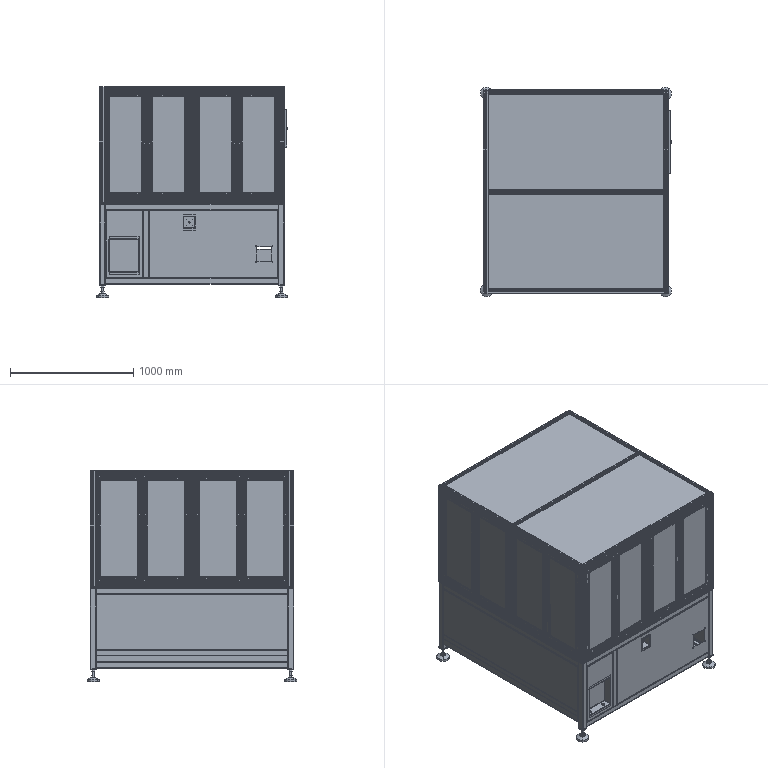Part | SolidWorks | features ReferencePattern 10, MirrorCompFeat 4 | 145 solids | 5501 faces | volume 100211807 mm3 | plane 3772 | cylinder 1465 | spline 136 | cone 128 | commonest cylinder face diameters 5 x268 3.3 x112 4.5 x112 6.5 x112 6 x108 2.2 x102